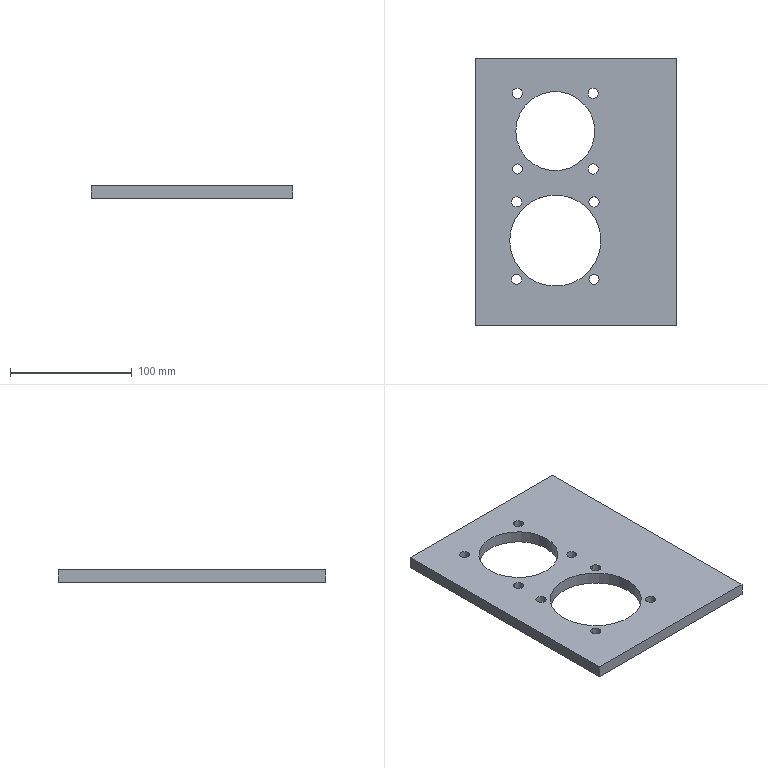Part | SolidWorks | features BaseBody 1 | 1 solid | 26 faces | box 166 x 220 x 10 mm | volume 283430 mm3 | cylinder 20 | plane 6 | commonest cylinder face diameters 8.376 x16 65 x2 75 x2
STEP:
#1=CARTESIAN_POINT('',(-32.665,-213.029,476.121));
#2=VERTEX_POINT('',#1);
#3=CARTESIAN_POINT('',(-107.665,-213.029,476.121));
#4=VERTEX_POINT('',#3);
#5=CARTESIAN_POINT('',(-70.165,-213.029,476.121));
#6=DIRECTION('',(0.,0.,-1.));
#7=DIRECTION('',(-1.,0.,0.));
#8=AXIS2_PLACEMENT_3D('',#5,#6,#7);
#9=CIRCLE('',#8,37.5);
#10=EDGE_CURVE('',#2,#4,#9,.T.);
#11=ORIENTED_EDGE('',*,*,#10,.F.);
#12=CARTESIAN_POINT('',(-32.665,-213.029,466.121));
#13=VERTEX_POINT('',#12);
#14=CARTESIAN_POINT('',(-32.665,-213.029,476.121));
#15=DIRECTION('',(0.,0.,-1.));
#16=VECTOR('',#15,1000.);
#17=LINE('',#14,#16);
#18=EDGE_CURVE('',#2,#13,#17,.T.);
#19=ORIENTED_EDGE('',*,*,#18,.T.);
#20=CARTESIAN_POINT('',(-107.665,-213.029,466.121));
#21=VERTEX_POINT('',#20);
#22=CARTESIAN_POINT('',(-70.165,-213.029,466.121));
#23=DIRECTION('',(0.,0.,-1.));
#24=DIRECTION('',(-1.,0.,0.));
#25=AXIS2_PLACEMENT_3D('',#22,#23,#24);
#26=CIRCLE('',#25,37.5);
#27=EDGE_CURVE('',#13,#21,#26,.T.);
#28=ORIENTED_EDGE('',*,*,#27,.T.);
#29=CARTESIAN_POINT('',(-107.665,-213.029,476.121));
#30=DIRECTION('',(0.,0.,-1.));
#31=VECTOR('',#30,1000.);
#32=LINE('',#29,#31);
#33=EDGE_CURVE('',#4,#21,#32,.T.);
#34=ORIENTED_EDGE('',*,*,#33,.F.);
#35=EDGE_LOOP('',(#11,#19,#28,#34));
#36=FACE_OUTER_BOUND('',#35,.T.);
#37=CARTESIAN_POINT('',(-70.165,-213.029,476.121));
#38=DIRECTION('',(0.,0.,-1.));
#39=DIRECTION('',(-1.,0.,0.));
#40=AXIS2_PLACEMENT_3D('',#37,#38,#39);
#41=CYLINDRICAL_SURFACE('',#40,37.5);
#42=ADVANCED_FACE('',(#36),#41,.F.);
#43=CARTESIAN_POINT('',(-37.665,-123.029,476.121));
#44=VERTEX_POINT('',#43);
#45=CARTESIAN_POINT('',(-102.665,-123.029,476.121));
#46=VERTEX_POINT('',#45);
#47=CARTESIAN_POINT('',(-70.165,-123.029,476.121));
#48=DIRECTION('',(0.,0.,-1.));
#49=DIRECTION('',(-1.,0.,0.));
#50=AXIS2_PLACEMENT_3D('',#47,#48,#49);
#51=CIRCLE('',#50,32.5);
#52=EDGE_CURVE('',#44,#46,#51,.T.);
#53=ORIENTED_EDGE('',*,*,#52,.F.);
#54=CARTESIAN_POINT('',(-37.665,-123.029,466.121));
#55=VERTEX_POINT('',#54);
#56=CARTESIAN_POINT('',(-37.665,-123.029,476.121));
#57=DIRECTION('',(0.,0.,-1.));
#58=VECTOR('',#57,1000.);
#59=LINE('',#56,#58);
#60=EDGE_CURVE('',#44,#55,#59,.T.);
#61=ORIENTED_EDGE('',*,*,#60,.T.);
#62=CARTESIAN_POINT('',(-102.665,-123.029,466.121));
#63=VERTEX_POINT('',#62);
#64=CARTESIAN_POINT('',(-70.165,-123.029,466.121));
#65=DIRECTION('',(0.,0.,-1.));
#66=DIRECTION('',(-1.,0.,0.));
#67=AXIS2_PLACEMENT_3D('',#64,#65,#66);
#68=CIRCLE('',#67,32.5);
#69=EDGE_CURVE('',#55,#63,#68,.T.);
#70=ORIENTED_EDGE('',*,*,#69,.T.);
#71=CARTESIAN_POINT('',(-102.665,-123.029,476.121));
#72=DIRECTION('',(0.,0.,-1.));
#73=VECTOR('',#72,1000.);
#74=LINE('',#71,#73);
#75=EDGE_CURVE('',#46,#63,#74,.T.);
#76=ORIENTED_EDGE('',*,*,#75,.F.);
#77=EDGE_LOOP('',(#53,#61,#70,#76));
#78=FACE_OUTER_BOUND('',#77,.T.);
#79=CARTESIAN_POINT('',(-70.165,-123.029,476.121));
#80=DIRECTION('',(0.,0.,-1.));
#81=DIRECTION('',(-1.,0.,0.));
#82=AXIS2_PLACEMENT_3D('',#79,#80,#81);
#83=CYLINDRICAL_SURFACE('',#82,32.5);
#84=ADVANCED_FACE('',(#78),#83,.F.);
#85=CARTESIAN_POINT('',(-39.052,-96.104,466.121));
#86=VERTEX_POINT('',#85);
#87=CARTESIAN_POINT('',(-39.052,-87.728,466.121));
#88=VERTEX_POINT('',#87);
#89=CARTESIAN_POINT('',(-39.052,-91.916,466.121));
#90=DIRECTION('',(0.,0.,-1.));
#91=DIRECTION('',(0.,-1.,0.));
#92=AXIS2_PLACEMENT_3D('',#89,#90,#91);
#93=CIRCLE('',#92,4.188);
#94=EDGE_CURVE('',#86,#88,#93,.T.);
#95=ORIENTED_EDGE('',*,*,#94,.T.);
#96=CARTESIAN_POINT('',(-39.052,-87.728,476.121));
#97=VERTEX_POINT('',#96);
#98=CARTESIAN_POINT('',(-39.052,-87.728,200.338));
#99=DIRECTION('',(0.,0.,1.));
#100=VECTOR('',#99,1000.);
#101=LINE('',#98,#100);
#102=EDGE_CURVE('',#88,#97,#101,.T.);
#103=ORIENTED_EDGE('',*,*,#102,.T.);
#104=CARTESIAN_POINT('',(-39.052,-96.104,476.121));
#105=VERTEX_POINT('',#104);
#106=CARTESIAN_POINT('',(-39.052,-91.916,476.121));
#107=DIRECTION('',(0.,0.,-1.));
#108=DIRECTION('',(0.,-1.,0.));
#109=AXIS2_PLACEMENT_3D('',#106,#107,#108);
#110=CIRCLE('',#109,4.188);
#111=EDGE_CURVE('',#105,#97,#110,.T.);
#112=ORIENTED_EDGE('',*,*,#111,.F.);
#113=CARTESIAN_POINT('',(-39.052,-96.104,200.338));
#114=DIRECTION('',(0.,0.,1.));
#115=VECTOR('',#114,1000.);
#116=LINE('',#113,#115);
#117=EDGE_CURVE('',#86,#105,#116,.T.);
#118=ORIENTED_EDGE('',*,*,#117,.F.);
#119=EDGE_LOOP('',(#95,#103,#112,#118));
#120=FACE_OUTER_BOUND('',#119,.T.);
#121=CARTESIAN_POINT('',(-39.052,-91.916,200.338));
#122=DIRECTION('',(0.,0.,1.));
#123=DIRECTION('',(0.,-1.,0.));
#124=AXIS2_PLACEMENT_3D('',#121,#122,#123);
#125=CYLINDRICAL_SURFACE('',#124,4.188);
#126=ADVANCED_FACE('',(#120),#125,.F.);
#127=CARTESIAN_POINT('',(-34.864,-154.141,466.121));
#128=VERTEX_POINT('',#127);
#129=CARTESIAN_POINT('',(-43.24,-154.141,466.121));
#130=VERTEX_POINT('',#129);
#131=CARTESIAN_POINT('',(-39.052,-154.141,466.121));
#132=DIRECTION('',(0.,0.,-1.));
#133=DIRECTION('',(1.,0.,0.));
#134=AXIS2_PLACEMENT_3D('',#131,#132,#133);
#135=CIRCLE('',#134,4.188);
#136=EDGE_CURVE('',#128,#130,#135,.T.);
#137=ORIENTED_EDGE('',*,*,#136,.T.);
#138=CARTESIAN_POINT('',(-43.24,-154.141,476.121));
#139=VERTEX_POINT('',#138);
#140=CARTESIAN_POINT('',(-43.24,-154.141,200.338));
#141=DIRECTION('',(0.,0.,1.));
#142=VECTOR('',#141,1000.);
#143=LINE('',#140,#142);
#144=EDGE_CURVE('',#130,#139,#143,.T.);
#145=ORIENTED_EDGE('',*,*,#144,.T.);
#146=CARTESIAN_POINT('',(-34.864,-154.141,476.121));
#147=VERTEX_POINT('',#146);
#148=CARTESIAN_POINT('',(-39.052,-154.141,476.121));
#149=DIRECTION('',(0.,0.,-1.));
#150=DIRECTION('',(1.,0.,0.));
#151=AXIS2_PLACEMENT_3D('',#148,#149,#150);
#152=CIRCLE('',#151,4.188);
#153=EDGE_CURVE('',#147,#139,#152,.T.);
#154=ORIENTED_EDGE('',*,*,#153,.F.);
#155=CARTESIAN_POINT('',(-34.864,-154.141,200.338));
#156=DIRECTION('',(0.,0.,1.));
#157=VECTOR('',#156,1000.);
#158=LINE('',#155,#157);
#159=EDGE_CURVE('',#128,#147,#158,.T.);
#160=ORIENTED_EDGE('',*,*,#159,.F.);
#161=EDGE_LOOP('',(#137,#145,#154,#160));
#162=FACE_OUTER_BOUND('',#161,.T.);
#163=CARTESIAN_POINT('',(-39.052,-154.141,200.338));
#164=DIRECTION('',(0.,0.,1.));
#165=DIRECTION('',(1.,0.,0.));
#166=AXIS2_PLACEMENT_3D('',#163,#164,#165);
#167=CYLINDRICAL_SURFACE('',#166,4.188);
#168=ADVANCED_FACE('',(#162),#167,.F.);
#169=CARTESIAN_POINT('',(-101.277,-158.329,466.121));
#170=VERTEX_POINT('',#169);
#171=CARTESIAN_POINT('',(-101.277,-149.953,466.121));
#172=VERTEX_POINT('',#171);
#173=CARTESIAN_POINT('',(-101.277,-154.141,466.121));
#174=DIRECTION('',(0.,0.,-1.));
#175=DIRECTION('',(0.,-1.,0.));
#176=AXIS2_PLACEMENT_3D('',#173,#174,#175);
#177=CIRCLE('',#176,4.188);
#178=EDGE_CURVE('',#170,#172,#177,.T.);
#179=ORIENTED_EDGE('',*,*,#178,.T.);
#180=CARTESIAN_POINT('',(-101.277,-149.953,476.121));
#181=VERTEX_POINT('',#180);
#182=CARTESIAN_POINT('',(-101.277,-149.953,200.338));
#183=DIRECTION('',(0.,0.,1.));
#184=VECTOR('',#183,1000.);
#185=LINE('',#182,#184);
#186=EDGE_CURVE('',#172,#181,#185,.T.);
#187=ORIENTED_EDGE('',*,*,#186,.T.);
#188=CARTESIAN_POINT('',(-101.277,-158.329,476.121));
#189=VERTEX_POINT('',#188);
#190=CARTESIAN_POINT('',(-101.277,-154.141,476.121));
#191=DIRECTION('',(0.,0.,-1.));
#192=DIRECTION('',(0.,-1.,0.));
#193=AXIS2_PLACEMENT_3D('',#190,#191,#192);
#194=CIRCLE('',#193,4.188);
#195=EDGE_CURVE('',#189,#181,#194,.T.);
#196=ORIENTED_EDGE('',*,*,#195,.F.);
#197=CARTESIAN_POINT('',(-101.277,-158.329,200.338));
#198=DIRECTION('',(0.,0.,1.));
#199=VECTOR('',#198,1000.);
#200=LINE('',#197,#199);
#201=EDGE_CURVE('',#170,#189,#200,.T.);
#202=ORIENTED_EDGE('',*,*,#201,.F.);
#203=EDGE_LOOP('',(#179,#187,#196,#202));
#204=FACE_OUTER_BOUND('',#203,.T.);
#205=CARTESIAN_POINT('',(-101.277,-154.141,200.338));
#206=DIRECTION('',(0.,0.,1.));
#207=DIRECTION('',(0.,-1.,0.));
#208=AXIS2_PLACEMENT_3D('',#205,#206,#207);
#209=CYLINDRICAL_SURFACE('',#208,4.188);
#210=ADVANCED_FACE('',(#204),#209,.F.);
#211=CARTESIAN_POINT('',(-97.089,-91.916,466.121));
#212=VERTEX_POINT('',#211);
#213=CARTESIAN_POINT('',(-105.465,-91.916,466.121));
#214=VERTEX_POINT('',#213);
#215=CARTESIAN_POINT('',(-101.277,-91.916,466.121));
#216=DIRECTION('',(0.,0.,-1.));
#217=DIRECTION('',(1.,0.,0.));
#218=AXIS2_PLACEMENT_3D('',#215,#216,#217);
#219=CIRCLE('',#218,4.188);
#220=EDGE_CURVE('',#212,#214,#219,.T.);
#221=ORIENTED_EDGE('',*,*,#220,.T.);
#222=CARTESIAN_POINT('',(-105.465,-91.916,476.121));
#223=VERTEX_POINT('',#222);
#224=CARTESIAN_POINT('',(-105.465,-91.916,200.338));
#225=DIRECTION('',(0.,0.,1.));
#226=VECTOR('',#225,1000.);
#227=LINE('',#224,#226);
#228=EDGE_CURVE('',#214,#223,#227,.T.);
#229=ORIENTED_EDGE('',*,*,#228,.T.);
#230=CARTESIAN_POINT('',(-97.089,-91.916,476.121));
#231=VERTEX_POINT('',#230);
#232=CARTESIAN_POINT('',(-101.277,-91.916,476.121));
#233=DIRECTION('',(0.,0.,-1.));
#234=DIRECTION('',(1.,0.,0.));
#235=AXIS2_PLACEMENT_3D('',#232,#233,#234);
#236=CIRCLE('',#235,4.188);
#237=EDGE_CURVE('',#231,#223,#236,.T.);
#238=ORIENTED_EDGE('',*,*,#237,.F.);
#239=CARTESIAN_POINT('',(-97.089,-91.916,200.338));
#240=DIRECTION('',(0.,0.,1.));
#241=VECTOR('',#240,1000.);
#242=LINE('',#239,#241);
#243=EDGE_CURVE('',#212,#231,#242,.T.);
#244=ORIENTED_EDGE('',*,*,#243,.F.);
#245=EDGE_LOOP('',(#221,#229,#238,#244));
#246=FACE_OUTER_BOUND('',#245,.T.);
#247=CARTESIAN_POINT('',(-101.277,-91.916,200.338));
#248=DIRECTION('',(0.,0.,1.));
#249=DIRECTION('',(1.,0.,0.));
#250=AXIS2_PLACEMENT_3D('',#247,#248,#249);
#251=CYLINDRICAL_SURFACE('',#250,4.188);
#252=ADVANCED_FACE('',(#246),#251,.F.);
#253=CARTESIAN_POINT('',(-38.345,-185.397,466.121));
#254=VERTEX_POINT('',#253);
#255=CARTESIAN_POINT('',(-38.345,-177.021,466.121));
#256=VERTEX_POINT('',#255);
#257=CARTESIAN_POINT('',(-38.345,-181.209,466.121));
#258=DIRECTION('',(0.,0.,-1.));
#259=DIRECTION('',(0.,-1.,0.));
#260=AXIS2_PLACEMENT_3D('',#257,#258,#259);
#261=CIRCLE('',#260,4.188);
#262=EDGE_CURVE('',#254,#256,#261,.T.);
#263=ORIENTED_EDGE('',*,*,#262,.T.);
#264=CARTESIAN_POINT('',(-38.345,-177.021,476.121));
#265=VERTEX_POINT('',#264);
#266=CARTESIAN_POINT('',(-38.345,-177.021,200.338));
#267=DIRECTION('',(0.,0.,1.));
#268=VECTOR('',#267,1000.);
#269=LINE('',#266,#268);
#270=EDGE_CURVE('',#256,#265,#269,.T.);
#271=ORIENTED_EDGE('',*,*,#270,.T.);
#272=CARTESIAN_POINT('',(-38.345,-185.397,476.121));
#273=VERTEX_POINT('',#272);
#274=CARTESIAN_POINT('',(-38.345,-181.209,476.121));
#275=DIRECTION('',(0.,0.,-1.));
#276=DIRECTION('',(0.,-1.,0.));
#277=AXIS2_PLACEMENT_3D('',#274,#275,#276);
#278=CIRCLE('',#277,4.188);
#279=EDGE_CURVE('',#273,#265,#278,.T.);
#280=ORIENTED_EDGE('',*,*,#279,.F.);
#281=CARTESIAN_POINT('',(-38.345,-185.397,200.338));
#282=DIRECTION('',(0.,0.,1.));
#283=VECTOR('',#282,1000.);
#284=LINE('',#281,#283);
#285=EDGE_CURVE('',#254,#273,#284,.T.);
#286=ORIENTED_EDGE('',*,*,#285,.F.);
#287=EDGE_LOOP('',(#263,#271,#280,#286));
#288=FACE_OUTER_BOUND('',#287,.T.);
#289=CARTESIAN_POINT('',(-38.345,-181.209,200.338));
#290=DIRECTION('',(0.,0.,1.));
#291=DIRECTION('',(0.,-1.,0.));
#292=AXIS2_PLACEMENT_3D('',#289,#290,#291);
#293=CYLINDRICAL_SURFACE('',#292,4.188);
#294=ADVANCED_FACE('',(#288),#293,.F.);
#295=CARTESIAN_POINT('',(-34.157,-244.848,466.121));
#296=VERTEX_POINT('',#295);
#297=CARTESIAN_POINT('',(-42.533,-244.848,466.121));
#298=VERTEX_POINT('',#297);
#299=CARTESIAN_POINT('',(-38.345,-244.848,466.121));
#300=DIRECTION('',(0.,0.,-1.));
#301=DIRECTION('',(1.,0.,0.));
#302=AXIS2_PLACEMENT_3D('',#299,#300,#301);
#303=CIRCLE('',#302,4.188);
#304=EDGE_CURVE('',#296,#298,#303,.T.);
#305=ORIENTED_EDGE('',*,*,#304,.T.);
#306=CARTESIAN_POINT('',(-42.533,-244.848,476.121));
#307=VERTEX_POINT('',#306);
#308=CARTESIAN_POINT('',(-42.533,-244.848,200.338));
#309=DIRECTION('',(0.,0.,1.));
#310=VECTOR('',#309,1000.);
#311=LINE('',#308,#310);
#312=EDGE_CURVE('',#298,#307,#311,.T.);
#313=ORIENTED_EDGE('',*,*,#312,.T.);
#314=CARTESIAN_POINT('',(-34.157,-244.848,476.121));
#315=VERTEX_POINT('',#314);
#316=CARTESIAN_POINT('',(-38.345,-244.848,476.121));
#317=DIRECTION('',(0.,0.,-1.));
#318=DIRECTION('',(1.,0.,0.));
#319=AXIS2_PLACEMENT_3D('',#316,#317,#318);
#320=CIRCLE('',#319,4.188);
#321=EDGE_CURVE('',#315,#307,#320,.T.);
#322=ORIENTED_EDGE('',*,*,#321,.F.);
#323=CARTESIAN_POINT('',(-34.157,-244.848,200.338));
#324=DIRECTION('',(0.,0.,1.));
#325=VECTOR('',#324,1000.);
#326=LINE('',#323,#325);
#327=EDGE_CURVE('',#296,#315,#326,.T.);
#328=ORIENTED_EDGE('',*,*,#327,.F.);
#329=EDGE_LOOP('',(#305,#313,#322,#328));
#330=FACE_OUTER_BOUND('',#329,.T.);
#331=CARTESIAN_POINT('',(-38.345,-244.848,200.338));
#332=DIRECTION('',(0.,0.,1.));
#333=DIRECTION('',(1.,0.,0.));
#334=AXIS2_PLACEMENT_3D('',#331,#332,#333);
#335=CYLINDRICAL_SURFACE('',#334,4.188);
#336=ADVANCED_FACE('',(#330),#335,.F.);
#337=CARTESIAN_POINT('',(-101.984,-249.036,466.121));
#338=VERTEX_POINT('',#337);
#339=CARTESIAN_POINT('',(-101.984,-240.66,466.121));
#340=VERTEX_POINT('',#339);
#341=CARTESIAN_POINT('',(-101.984,-244.848,466.121));
#342=DIRECTION('',(0.,0.,-1.));
#343=DIRECTION('',(0.,-1.,0.));
#344=AXIS2_PLACEMENT_3D('',#341,#342,#343);
#345=CIRCLE('',#344,4.188);
#346=EDGE_CURVE('',#338,#340,#345,.T.);
#347=ORIENTED_EDGE('',*,*,#346,.T.);
#348=CARTESIAN_POINT('',(-101.984,-240.66,476.121));
#349=VERTEX_POINT('',#348);
#350=CARTESIAN_POINT('',(-101.984,-240.66,200.338));
#351=DIRECTION('',(0.,0.,1.));
#352=VECTOR('',#351,1000.);
#353=LINE('',#350,#352);
#354=EDGE_CURVE('',#340,#349,#353,.T.);
#355=ORIENTED_EDGE('',*,*,#354,.T.);
#356=CARTESIAN_POINT('',(-101.984,-249.036,476.121));
#357=VERTEX_POINT('',#356);
#358=CARTESIAN_POINT('',(-101.984,-244.848,476.121));
#359=DIRECTION('',(0.,0.,-1.));
#360=DIRECTION('',(0.,-1.,0.));
#361=AXIS2_PLACEMENT_3D('',#358,#359,#360);
#362=CIRCLE('',#361,4.188);
#363=EDGE_CURVE('',#357,#349,#362,.T.);
#364=ORIENTED_EDGE('',*,*,#363,.F.);
#365=CARTESIAN_POINT('',(-101.984,-249.036,200.338));
#366=DIRECTION('',(0.,0.,1.));
#367=VECTOR('',#366,1000.);
#368=LINE('',#365,#367);
#369=EDGE_CURVE('',#338,#357,#368,.T.);
#370=ORIENTED_EDGE('',*,*,#369,.F.);
#371=EDGE_LOOP('',(#347,#355,#364,#370));
#372=FACE_OUTER_BOUND('',#371,.T.);
#373=CARTESIAN_POINT('',(-101.984,-244.848,200.338));
#374=DIRECTION('',(0.,0.,1.));
#375=DIRECTION('',(0.,-1.,0.));
#376=AXIS2_PLACEMENT_3D('',#373,#374,#375);
#377=CYLINDRICAL_SURFACE('',#376,4.188);
#378=ADVANCED_FACE('',(#372),#377,.F.);
#379=CARTESIAN_POINT('',(-97.796,-181.209,466.121));
#380=VERTEX_POINT('',#379);
#381=CARTESIAN_POINT('',(-106.172,-181.209,466.121));
#382=VERTEX_POINT('',#381);
#383=CARTESIAN_POINT('',(-101.984,-181.209,466.121));
#384=DIRECTION('',(0.,0.,-1.));
#385=DIRECTION('',(1.,0.,0.));
#386=AXIS2_PLACEMENT_3D('',#383,#384,#385);
#387=CIRCLE('',#386,4.188);
#388=EDGE_CURVE('',#380,#382,#387,.T.);
#389=ORIENTED_EDGE('',*,*,#388,.T.);
#390=CARTESIAN_POINT('',(-106.172,-181.209,476.121));
#391=VERTEX_POINT('',#390);
#392=CARTESIAN_POINT('',(-106.172,-181.209,200.338));
#393=DIRECTION('',(0.,0.,1.));
#394=VECTOR('',#393,1000.);
#395=LINE('',#392,#394);
#396=EDGE_CURVE('',#382,#391,#395,.T.);
#397=ORIENTED_EDGE('',*,*,#396,.T.);
#398=CARTESIAN_POINT('',(-97.796,-181.209,476.121));
#399=VERTEX_POINT('',#398);
#400=CARTESIAN_POINT('',(-101.984,-181.209,476.121));
#401=DIRECTION('',(0.,0.,-1.));
#402=DIRECTION('',(1.,0.,0.));
#403=AXIS2_PLACEMENT_3D('',#400,#401,#402);
#404=CIRCLE('',#403,4.188);
#405=EDGE_CURVE('',#399,#391,#404,.T.);
#406=ORIENTED_EDGE('',*,*,#405,.F.);
#407=CARTESIAN_POINT('',(-97.796,-181.209,200.338));
#408=DIRECTION('',(0.,0.,1.));
#409=VECTOR('',#408,1000.);
#410=LINE('',#407,#409);
#411=EDGE_CURVE('',#380,#399,#410,.T.);
#412=ORIENTED_EDGE('',*,*,#411,.F.);
#413=EDGE_LOOP('',(#389,#397,#406,#412));
#414=FACE_OUTER_BOUND('',#413,.T.);
#415=CARTESIAN_POINT('',(-101.984,-181.209,200.338));
#416=DIRECTION('',(0.,0.,1.));
#417=DIRECTION('',(1.,0.,0.));
#418=AXIS2_PLACEMENT_3D('',#415,#416,#417);
#419=CYLINDRICAL_SURFACE('',#418,4.188);
#420=ADVANCED_FACE('',(#414),#419,.F.);
#421=CARTESIAN_POINT('',(-70.165,-213.029,466.121));
#422=DIRECTION('',(0.,0.,-1.));
#423=DIRECTION('',(-1.,0.,0.));
#424=AXIS2_PLACEMENT_3D('',#421,#422,#423);
#425=CIRCLE('',#424,37.5);
#426=EDGE_CURVE('',#21,#13,#425,.T.);
#427=ORIENTED_EDGE('',*,*,#426,.F.);
#428=ORIENTED_EDGE('',*,*,#27,.F.);
#429=EDGE_LOOP('',(#427,#428));
#430=FACE_BOUND('',#429,.T.);
#431=CARTESIAN_POINT('',(-70.165,-123.029,466.121));
#432=DIRECTION('',(0.,0.,-1.));
#433=DIRECTION('',(-1.,0.,0.));
#434=AXIS2_PLACEMENT_3D('',#431,#432,#433);
#435=CIRCLE('',#434,32.5);
#436=EDGE_CURVE('',#63,#55,#435,.T.);
#437=ORIENTED_EDGE('',*,*,#436,.F.);
#438=ORIENTED_EDGE('',*,*,#69,.F.);
#439=EDGE_LOOP('',(#437,#438));
#440=FACE_BOUND('',#439,.T.);
#441=ORIENTED_EDGE('',*,*,#94,.F.);
#442=CARTESIAN_POINT('',(-39.052,-91.916,466.121));
#443=DIRECTION('',(0.,0.,-1.));
#444=DIRECTION('',(0.,-1.,0.));
#445=AXIS2_PLACEMENT_3D('',#442,#443,#444);
#446=CIRCLE('',#445,4.188);
#447=EDGE_CURVE('',#88,#86,#446,.T.);
#448=ORIENTED_EDGE('',*,*,#447,.F.);
#449=EDGE_LOOP('',(#441,#448));
#450=FACE_BOUND('',#449,.T.);
#451=ORIENTED_EDGE('',*,*,#136,.F.);
#452=CARTESIAN_POINT('',(-39.052,-154.141,466.121));
#453=DIRECTION('',(0.,0.,-1.));
#454=DIRECTION('',(1.,0.,0.));
#455=AXIS2_PLACEMENT_3D('',#452,#453,#454);
#456=CIRCLE('',#455,4.188);
#457=EDGE_CURVE('',#130,#128,#456,.T.);
#458=ORIENTED_EDGE('',*,*,#457,.F.);
#459=EDGE_LOOP('',(#451,#458));
#460=FACE_BOUND('',#459,.T.);
#461=ORIENTED_EDGE('',*,*,#178,.F.);
#462=CARTESIAN_POINT('',(-101.277,-154.141,466.121));
#463=DIRECTION('',(0.,0.,-1.));
#464=DIRECTION('',(0.,-1.,0.));
#465=AXIS2_PLACEMENT_3D('',#462,#463,#464);
#466=CIRCLE('',#465,4.188);
#467=EDGE_CURVE('',#172,#170,#466,.T.);
#468=ORIENTED_EDGE('',*,*,#467,.F.);
#469=EDGE_LOOP('',(#461,#468));
#470=FACE_BOUND('',#469,.T.);
#471=ORIENTED_EDGE('',*,*,#220,.F.);
#472=CARTESIAN_POINT('',(-101.277,-91.916,466.121));
#473=DIRECTION('',(0.,0.,-1.));
#474=DIRECTION('',(1.,0.,0.));
#475=AXIS2_PLACEMENT_3D('',#472,#473,#474);
#476=CIRCLE('',#475,4.188);
#477=EDGE_CURVE('',#214,#212,#476,.T.);
#478=ORIENTED_EDGE('',*,*,#477,.F.);
#479=EDGE_LOOP('',(#471,#478));
#480=FACE_BOUND('',#479,.T.);
#481=ORIENTED_EDGE('',*,*,#262,.F.);
#482=CARTESIAN_POINT('',(-38.345,-181.209,466.121));
#483=DIRECTION('',(0.,0.,-1.));
#484=DIRECTION('',(0.,-1.,0.));
#485=AXIS2_PLACEMENT_3D('',#482,#483,#484);
#486=CIRCLE('',#485,4.188);
#487=EDGE_CURVE('',#256,#254,#486,.T.);
#488=ORIENTED_EDGE('',*,*,#487,.F.);
#489=EDGE_LOOP('',(#481,#488));
#490=FACE_BOUND('',#489,.T.);
#491=ORIENTED_EDGE('',*,*,#304,.F.);
#492=CARTESIAN_POINT('',(-38.345,-244.848,466.121));
#493=DIRECTION('',(0.,0.,-1.));
#494=DIRECTION('',(1.,0.,0.));
#495=AXIS2_PLACEMENT_3D('',#492,#493,#494);
#496=CIRCLE('',#495,4.188);
#497=EDGE_CURVE('',#298,#296,#496,.T.);
#498=ORIENTED_EDGE('',*,*,#497,.F.);
#499=EDGE_LOOP('',(#491,#498));
#500=FACE_BOUND('',#499,.T.);
#501=ORIENTED_EDGE('',*,*,#346,.F.);
#502=CARTESIAN_POINT('',(-101.984,-244.848,466.121));
#503=DIRECTION('',(0.,0.,-1.));
#504=DIRECTION('',(0.,-1.,0.));
#505=AXIS2_PLACEMENT_3D('',#502,#503,#504);
#506=CIRCLE('',#505,4.188);
#507=EDGE_CURVE('',#340,#338,#506,.T.);
#508=ORIENTED_EDGE('',*,*,#507,.F.);
#509=EDGE_LOOP('',(#501,#508));
#510=FACE_BOUND('',#509,.T.);
#511=ORIENTED_EDGE('',*,*,#388,.F.);
#512=CARTESIAN_POINT('',(-101.984,-181.209,466.121));
#513=DIRECTION('',(0.,0.,-1.));
#514=DIRECTION('',(1.,0.,0.));
#515=AXIS2_PLACEMENT_3D('',#512,#513,#514);
#516=CIRCLE('',#515,4.188);
#517=EDGE_CURVE('',#382,#380,#516,.T.);
#518=ORIENTED_EDGE('',*,*,#517,.F.);
#519=EDGE_LOOP('',(#511,#518));
#520=FACE_BOUND('',#519,.T.);
#521=CARTESIAN_POINT('',(-136.165,-283.029,466.121));
#522=VERTEX_POINT('',#521);
#523=CARTESIAN_POINT('',(29.835,-283.029,466.121));
#524=VERTEX_POINT('',#523);
#525=CARTESIAN_POINT('',(-53.165,-283.029,466.121));
#526=DIRECTION('',(1.,0.,0.));
#527=VECTOR('',#526,1000.);
#528=LINE('',#525,#527);
#529=EDGE_CURVE('',#522,#524,#528,.T.);
#530=ORIENTED_EDGE('',*,*,#529,.F.);
#531=CARTESIAN_POINT('',(-136.165,-63.029,466.121));
#532=VERTEX_POINT('',#531);
#533=CARTESIAN_POINT('',(-136.165,-173.029,466.121));
#534=DIRECTION('',(0.,-1.,0.));
#535=VECTOR('',#534,1000.);
#536=LINE('',#533,#535);
#537=EDGE_CURVE('',#532,#522,#536,.T.);
#538=ORIENTED_EDGE('',*,*,#537,.F.);
#539=CARTESIAN_POINT('',(29.835,-63.029,466.121));
#540=VERTEX_POINT('',#539);
#541=CARTESIAN_POINT('',(-53.165,-63.029,466.121));
#542=DIRECTION('',(-1.,0.,0.));
#543=VECTOR('',#542,1000.);
#544=LINE('',#541,#543);
#545=EDGE_CURVE('',#540,#532,#544,.T.);
#546=ORIENTED_EDGE('',*,*,#545,.F.);
#547=CARTESIAN_POINT('',(29.835,-173.029,466.121));
#548=DIRECTION('',(0.,1.,0.));
#549=VECTOR('',#548,1000.);
#550=LINE('',#547,#549);
#551=EDGE_CURVE('',#524,#540,#550,.T.);
#552=ORIENTED_EDGE('',*,*,#551,.F.);
#553=EDGE_LOOP('',(#530,#538,#546,#552));
#554=FACE_OUTER_BOUND('',#553,.T.);
#555=CARTESIAN_POINT('',(-53.165,-173.029,466.121));
#556=DIRECTION('',(0.,0.,1.));
#557=DIRECTION('',(0.,-1.,0.));
#558=AXIS2_PLACEMENT_3D('',#555,#556,#557);
#559=PLANE('',#558);
#560=ADVANCED_FACE('',(#430,#440,#450,#460,#470,#480,#490,#500,#510,#520,#554),#559,.F.);
#561=ORIENTED_EDGE('',*,*,#18,.F.);
#562=CARTESIAN_POINT('',(-70.165,-213.029,476.121));
#563=DIRECTION('',(0.,0.,-1.));
#564=DIRECTION('',(-1.,0.,0.));
#565=AXIS2_PLACEMENT_3D('',#562,#563,#564);
#566=CIRCLE('',#565,37.5);
#567=EDGE_CURVE('',#4,#2,#566,.T.);
#568=ORIENTED_EDGE('',*,*,#567,.F.);
#569=ORIENTED_EDGE('',*,*,#33,.T.);
#570=ORIENTED_EDGE('',*,*,#426,.T.);
#571=EDGE_LOOP('',(#561,#568,#569,#570));
#572=FACE_OUTER_BOUND('',#571,.T.);
#573=CARTESIAN_POINT('',(-70.165,-213.029,476.121));
#574=DIRECTION('',(0.,0.,-1.));
#575=DIRECTION('',(-1.,0.,0.));
#576=AXIS2_PLACEMENT_3D('',#573,#574,#575);
#577=CYLINDRICAL_SURFACE('',#576,37.5);
#578=ADVANCED_FACE('',(#572),#577,.F.);
#579=ORIENTED_EDGE('',*,*,#60,.F.);
#580=CARTESIAN_POINT('',(-70.165,-123.029,476.121));
#581=DIRECTION('',(0.,0.,-1.));
#582=DIRECTION('',(-1.,0.,0.));
#583=AXIS2_PLACEMENT_3D('',#580,#581,#582);
#584=CIRCLE('',#583,32.5);
#585=EDGE_CURVE('',#46,#44,#584,.T.);
#586=ORIENTED_EDGE('',*,*,#585,.F.);
#587=ORIENTED_EDGE('',*,*,#75,.T.);
#588=ORIENTED_EDGE('',*,*,#436,.T.);
#589=EDGE_LOOP('',(#579,#586,#587,#588));
#590=FACE_OUTER_BOUND('',#589,.T.);
#591=CARTESIAN_POINT('',(-70.165,-123.029,476.121));
#592=DIRECTION('',(0.,0.,-1.));
#593=DIRECTION('',(-1.,0.,0.));
#594=AXIS2_PLACEMENT_3D('',#591,#592,#593);
#595=CYLINDRICAL_SURFACE('',#594,32.5);
#596=ADVANCED_FACE('',(#590),#595,.F.);
#597=ORIENTED_EDGE('',*,*,#102,.F.);
#598=ORIENTED_EDGE('',*,*,#447,.T.);
#599=ORIENTED_EDGE('',*,*,#117,.T.);
#600=CARTESIAN_POINT('',(-39.052,-91.916,476.121));
#601=DIRECTION('',(0.,0.,-1.));
#602=DIRECTION('',(0.,-1.,0.));
#603=AXIS2_PLACEMENT_3D('',#600,#601,#602);
#604=CIRCLE('',#603,4.188);
#605=EDGE_CURVE('',#97,#105,#604,.T.);
#606=ORIENTED_EDGE('',*,*,#605,.F.);
#607=EDGE_LOOP('',(#597,#598,#599,#606));
#608=FACE_OUTER_BOUND('',#607,.T.);
#609=CARTESIAN_POINT('',(-39.052,-91.916,200.338));
#610=DIRECTION('',(0.,0.,1.));
#611=DIRECTION('',(0.,-1.,0.));
#612=AXIS2_PLACEMENT_3D('',#609,#610,#611);
#613=CYLINDRICAL_SURFACE('',#612,4.188);
#614=ADVANCED_FACE('',(#608),#613,.F.);
#615=ORIENTED_EDGE('',*,*,#144,.F.);
#616=ORIENTED_EDGE('',*,*,#457,.T.);
#617=ORIENTED_EDGE('',*,*,#159,.T.);
#618=CARTESIAN_POINT('',(-39.052,-154.141,476.121));
#619=DIRECTION('',(0.,0.,-1.));
#620=DIRECTION('',(1.,0.,0.));
#621=AXIS2_PLACEMENT_3D('',#618,#619,#620);
#622=CIRCLE('',#621,4.188);
#623=EDGE_CURVE('',#139,#147,#622,.T.);
#624=ORIENTED_EDGE('',*,*,#623,.F.);
#625=EDGE_LOOP('',(#615,#616,#617,#624));
#626=FACE_OUTER_BOUND('',#625,.T.);
#627=CARTESIAN_POINT('',(-39.052,-154.141,200.338));
#628=DIRECTION('',(0.,0.,1.));
#629=DIRECTION('',(1.,0.,0.));
#630=AXIS2_PLACEMENT_3D('',#627,#628,#629);
#631=CYLINDRICAL_SURFACE('',#630,4.188);
#632=ADVANCED_FACE('',(#626),#631,.F.);
#633=ORIENTED_EDGE('',*,*,#186,.F.);
#634=ORIENTED_EDGE('',*,*,#467,.T.);
#635=ORIENTED_EDGE('',*,*,#201,.T.);
#636=CARTESIAN_POINT('',(-101.277,-154.141,476.121));
#637=DIRECTION('',(0.,0.,-1.));
#638=DIRECTION('',(0.,-1.,0.));
#639=AXIS2_PLACEMENT_3D('',#636,#637,#638);
#640=CIRCLE('',#639,4.188);
#641=EDGE_CURVE('',#181,#189,#640,.T.);
#642=ORIENTED_EDGE('',*,*,#641,.F.);
#643=EDGE_LOOP('',(#633,#634,#635,#642));
#644=FACE_OUTER_BOUND('',#643,.T.);
#645=CARTESIAN_POINT('',(-101.277,-154.141,200.338));
#646=DIRECTION('',(0.,0.,1.));
#647=DIRECTION('',(0.,-1.,0.));
#648=AXIS2_PLACEMENT_3D('',#645,#646,#647);
#649=CYLINDRICAL_SURFACE('',#648,4.188);
#650=ADVANCED_FACE('',(#644),#649,.F.);
#651=ORIENTED_EDGE('',*,*,#228,.F.);
#652=ORIENTED_EDGE('',*,*,#477,.T.);
#653=ORIENTED_EDGE('',*,*,#243,.T.);
#654=CARTESIAN_POINT('',(-101.277,-91.916,476.121));
#655=DIRECTION('',(0.,0.,-1.));
#656=DIRECTION('',(1.,0.,0.));
#657=AXIS2_PLACEMENT_3D('',#654,#655,#656);
#658=CIRCLE('',#657,4.188);
#659=EDGE_CURVE('',#223,#231,#658,.T.);
#660=ORIENTED_EDGE('',*,*,#659,.F.);
#661=EDGE_LOOP('',(#651,#652,#653,#660));
#662=FACE_OUTER_BOUND('',#661,.T.);
#663=CARTESIAN_POINT('',(-101.277,-91.916,200.338));
#664=DIRECTION('',(0.,0.,1.));
#665=DIRECTION('',(1.,0.,0.));
#666=AXIS2_PLACEMENT_3D('',#663,#664,#665);
#667=CYLINDRICAL_SURFACE('',#666,4.188);
#668=ADVANCED_FACE('',(#662),#667,.F.);
#669=ORIENTED_EDGE('',*,*,#270,.F.);
#670=ORIENTED_EDGE('',*,*,#487,.T.);
#671=ORIENTED_EDGE('',*,*,#285,.T.);
#672=CARTESIAN_POINT('',(-38.345,-181.209,476.121));
#673=DIRECTION('',(0.,0.,-1.));
#674=DIRECTION('',(0.,-1.,0.));
#675=AXIS2_PLACEMENT_3D('',#672,#673,#674);
#676=CIRCLE('',#675,4.188);
#677=EDGE_CURVE('',#265,#273,#676,.T.);
#678=ORIENTED_EDGE('',*,*,#677,.F.);
#679=EDGE_LOOP('',(#669,#670,#671,#678));
#680=FACE_OUTER_BOUND('',#679,.T.);
#681=CARTESIAN_POINT('',(-38.345,-181.209,200.338));
#682=DIRECTION('',(0.,0.,1.));
#683=DIRECTION('',(0.,-1.,0.));
#684=AXIS2_PLACEMENT_3D('',#681,#682,#683);
#685=CYLINDRICAL_SURFACE('',#684,4.188);
#686=ADVANCED_FACE('',(#680),#685,.F.);
#687=ORIENTED_EDGE('',*,*,#312,.F.);
#688=ORIENTED_EDGE('',*,*,#497,.T.);
#689=ORIENTED_EDGE('',*,*,#327,.T.);
#690=CARTESIAN_POINT('',(-38.345,-244.848,476.121));
#691=DIRECTION('',(0.,0.,-1.));
#692=DIRECTION('',(1.,0.,0.));
#693=AXIS2_PLACEMENT_3D('',#690,#691,#692);
#694=CIRCLE('',#693,4.188);
#695=EDGE_CURVE('',#307,#315,#694,.T.);
#696=ORIENTED_EDGE('',*,*,#695,.F.);
#697=EDGE_LOOP('',(#687,#688,#689,#696));
#698=FACE_OUTER_BOUND('',#697,.T.);
#699=CARTESIAN_POINT('',(-38.345,-244.848,200.338));
#700=DIRECTION('',(0.,0.,1.));
#701=DIRECTION('',(1.,0.,0.));
#702=AXIS2_PLACEMENT_3D('',#699,#700,#701);
#703=CYLINDRICAL_SURFACE('',#702,4.188);
#704=ADVANCED_FACE('',(#698),#703,.F.);
#705=ORIENTED_EDGE('',*,*,#354,.F.);
#706=ORIENTED_EDGE('',*,*,#507,.T.);
#707=ORIENTED_EDGE('',*,*,#369,.T.);
#708=CARTESIAN_POINT('',(-101.984,-244.848,476.121));
#709=DIRECTION('',(0.,0.,-1.));
#710=DIRECTION('',(0.,-1.,0.));
#711=AXIS2_PLACEMENT_3D('',#708,#709,#710);
#712=CIRCLE('',#711,4.188);
#713=EDGE_CURVE('',#349,#357,#712,.T.);
#714=ORIENTED_EDGE('',*,*,#713,.F.);
#715=EDGE_LOOP('',(#705,#706,#707,#714));
#716=FACE_OUTER_BOUND('',#715,.T.);
#717=CARTESIAN_POINT('',(-101.984,-244.848,200.338));
#718=DIRECTION('',(0.,0.,1.));
#719=DIRECTION('',(0.,-1.,0.));
#720=AXIS2_PLACEMENT_3D('',#717,#718,#719);
#721=CYLINDRICAL_SURFACE('',#720,4.188);
#722=ADVANCED_FACE('',(#716),#721,.F.);
#723=ORIENTED_EDGE('',*,*,#396,.F.);
#724=ORIENTED_EDGE('',*,*,#517,.T.);
#725=ORIENTED_EDGE('',*,*,#411,.T.);
#726=CARTESIAN_POINT('',(-101.984,-181.209,476.121));
#727=DIRECTION('',(0.,0.,-1.));
#728=DIRECTION('',(1.,0.,0.));
#729=AXIS2_PLACEMENT_3D('',#726,#727,#728);
#730=CIRCLE('',#729,4.188);
#731=EDGE_CURVE('',#391,#399,#730,.T.);
#732=ORIENTED_EDGE('',*,*,#731,.F.);
#733=EDGE_LOOP('',(#723,#724,#725,#732));
#734=FACE_OUTER_BOUND('',#733,.T.);
#735=CARTESIAN_POINT('',(-101.984,-181.209,200.338));
#736=DIRECTION('',(0.,0.,1.));
#737=DIRECTION('',(1.,0.,0.));
#738=AXIS2_PLACEMENT_3D('',#735,#736,#737);
#739=CYLINDRICAL_SURFACE('',#738,4.188);
#740=ADVANCED_FACE('',(#734),#739,.F.);
#741=ORIENTED_EDGE('',*,*,#551,.T.);
#742=CARTESIAN_POINT('',(29.835,-63.029,476.121));
#743=VERTEX_POINT('',#742);
#744=CARTESIAN_POINT('',(29.835,-63.029,466.121));
#745=DIRECTION('',(0.,0.,1.));
#746=VECTOR('',#745,1000.);
#747=LINE('',#744,#746);
#748=EDGE_CURVE('',#540,#743,#747,.T.);
#749=ORIENTED_EDGE('',*,*,#748,.T.);
#750=CARTESIAN_POINT('',(29.835,-283.029,476.121));
#751=VERTEX_POINT('',#750);
#752=CARTESIAN_POINT('',(29.835,-63.029,476.121));
#753=DIRECTION('',(0.,-1.,0.));
#754=VECTOR('',#753,1000.);
#755=LINE('',#752,#754);
#756=EDGE_CURVE('',#743,#751,#755,.T.);
#757=ORIENTED_EDGE('',*,*,#756,.T.);
#758=CARTESIAN_POINT('',(29.835,-283.029,466.121));
#759=DIRECTION('',(0.,0.,-1.));
#760=VECTOR('',#759,1000.);
#761=LINE('',#758,#760);
#762=EDGE_CURVE('',#751,#524,#761,.T.);
#763=ORIENTED_EDGE('',*,*,#762,.T.);
#764=EDGE_LOOP('',(#741,#749,#757,#763));
#765=FACE_OUTER_BOUND('',#764,.T.);
#766=CARTESIAN_POINT('',(29.835,-63.029,466.121));
#767=DIRECTION('',(1.,0.,0.));
#768=DIRECTION('',(0.,0.,-1.));
#769=AXIS2_PLACEMENT_3D('',#766,#767,#768);
#770=PLANE('',#769);
#771=ADVANCED_FACE('',(#765),#770,.T.);
#772=ORIENTED_EDGE('',*,*,#529,.T.);
#773=ORIENTED_EDGE('',*,*,#762,.F.);
#774=CARTESIAN_POINT('',(-136.165,-283.029,476.121));
#775=VERTEX_POINT('',#774);
#776=CARTESIAN_POINT('',(29.835,-283.029,476.121));
#777=DIRECTION('',(-1.,0.,0.));
#778=VECTOR('',#777,1000.);
#779=LINE('',#776,#778);
#780=EDGE_CURVE('',#751,#775,#779,.T.);
#781=ORIENTED_EDGE('',*,*,#780,.T.);
#782=CARTESIAN_POINT('',(-136.165,-283.029,466.121));
#783=DIRECTION('',(0.,0.,-1.));
#784=VECTOR('',#783,1000.);
#785=LINE('',#782,#784);
#786=EDGE_CURVE('',#775,#522,#785,.T.);
#787=ORIENTED_EDGE('',*,*,#786,.T.);
#788=EDGE_LOOP('',(#772,#773,#781,#787));
#789=FACE_OUTER_BOUND('',#788,.T.);
#790=CARTESIAN_POINT('',(29.835,-283.029,466.121));
#791=DIRECTION('',(0.,-1.,0.));
#792=DIRECTION('',(0.,0.,-1.));
#793=AXIS2_PLACEMENT_3D('',#790,#791,#792);
#794=PLANE('',#793);
#795=ADVANCED_FACE('',(#789),#794,.T.);
#796=ORIENTED_EDGE('',*,*,#537,.T.);
#797=ORIENTED_EDGE('',*,*,#786,.F.);
#798=CARTESIAN_POINT('',(-136.165,-63.029,476.121));
#799=VERTEX_POINT('',#798);
#800=CARTESIAN_POINT('',(-136.165,-283.029,476.121));
#801=DIRECTION('',(0.,1.,0.));
#802=VECTOR('',#801,1000.);
#803=LINE('',#800,#802);
#804=EDGE_CURVE('',#775,#799,#803,.T.);
#805=ORIENTED_EDGE('',*,*,#804,.T.);
#806=CARTESIAN_POINT('',(-136.165,-63.029,466.121));
#807=DIRECTION('',(0.,0.,-1.));
#808=VECTOR('',#807,1000.);
#809=LINE('',#806,#808);
#810=EDGE_CURVE('',#799,#532,#809,.T.);
#811=ORIENTED_EDGE('',*,*,#810,.T.);
#812=EDGE_LOOP('',(#796,#797,#805,#811));
#813=FACE_OUTER_BOUND('',#812,.T.);
#814=CARTESIAN_POINT('',(-136.165,-283.029,466.121));
#815=DIRECTION('',(-1.,0.,0.));
#816=DIRECTION('',(0.,0.,1.));
#817=AXIS2_PLACEMENT_3D('',#814,#815,#816);
#818=PLANE('',#817);
#819=ADVANCED_FACE('',(#813),#818,.T.);
#820=ORIENTED_EDGE('',*,*,#545,.T.);
#821=ORIENTED_EDGE('',*,*,#810,.F.);
#822=CARTESIAN_POINT('',(-136.165,-63.029,476.121));
#823=DIRECTION('',(1.,0.,0.));
#824=VECTOR('',#823,1000.);
#825=LINE('',#822,#824);
#826=EDGE_CURVE('',#799,#743,#825,.T.);
#827=ORIENTED_EDGE('',*,*,#826,.T.);
#828=ORIENTED_EDGE('',*,*,#748,.F.);
#829=EDGE_LOOP('',(#820,#821,#827,#828));
#830=FACE_OUTER_BOUND('',#829,.T.);
#831=CARTESIAN_POINT('',(-136.165,-63.029,466.121));
#832=DIRECTION('',(0.,1.,0.));
#833=DIRECTION('',(0.,0.,1.));
#834=AXIS2_PLACEMENT_3D('',#831,#832,#833);
#835=PLANE('',#834);
#836=ADVANCED_FACE('',(#830),#835,.T.);
#837=ORIENTED_EDGE('',*,*,#567,.T.);
#838=ORIENTED_EDGE('',*,*,#10,.T.);
#839=EDGE_LOOP('',(#837,#838));
#840=FACE_BOUND('',#839,.T.);
#841=ORIENTED_EDGE('',*,*,#585,.T.);
#842=ORIENTED_EDGE('',*,*,#52,.T.);
#843=EDGE_LOOP('',(#841,#842));
#844=FACE_BOUND('',#843,.T.);
#845=ORIENTED_EDGE('',*,*,#111,.T.);
#846=ORIENTED_EDGE('',*,*,#605,.T.);
#847=EDGE_LOOP('',(#845,#846));
#848=FACE_BOUND('',#847,.T.);
#849=ORIENTED_EDGE('',*,*,#153,.T.);
#850=ORIENTED_EDGE('',*,*,#623,.T.);
#851=EDGE_LOOP('',(#849,#850));
#852=FACE_BOUND('',#851,.T.);
#853=ORIENTED_EDGE('',*,*,#195,.T.);
#854=ORIENTED_EDGE('',*,*,#641,.T.);
#855=EDGE_LOOP('',(#853,#854));
#856=FACE_BOUND('',#855,.T.);
#857=ORIENTED_EDGE('',*,*,#237,.T.);
#858=ORIENTED_EDGE('',*,*,#659,.T.);
#859=EDGE_LOOP('',(#857,#858));
#860=FACE_BOUND('',#859,.T.);
#861=ORIENTED_EDGE('',*,*,#279,.T.);
#862=ORIENTED_EDGE('',*,*,#677,.T.);
#863=EDGE_LOOP('',(#861,#862));
#864=FACE_BOUND('',#863,.T.);
#865=ORIENTED_EDGE('',*,*,#321,.T.);
#866=ORIENTED_EDGE('',*,*,#695,.T.);
#867=EDGE_LOOP('',(#865,#866));
#868=FACE_BOUND('',#867,.T.);
#869=ORIENTED_EDGE('',*,*,#363,.T.);
#870=ORIENTED_EDGE('',*,*,#713,.T.);
#871=EDGE_LOOP('',(#869,#870));
#872=FACE_BOUND('',#871,.T.);
#873=ORIENTED_EDGE('',*,*,#405,.T.);
#874=ORIENTED_EDGE('',*,*,#731,.T.);
#875=EDGE_LOOP('',(#873,#874));
#876=FACE_BOUND('',#875,.T.);
#877=ORIENTED_EDGE('',*,*,#826,.F.);
#878=ORIENTED_EDGE('',*,*,#804,.F.);
#879=ORIENTED_EDGE('',*,*,#780,.F.);
#880=ORIENTED_EDGE('',*,*,#756,.F.);
#881=EDGE_LOOP('',(#877,#878,#879,#880));
#882=FACE_OUTER_BOUND('',#881,.T.);
#883=CARTESIAN_POINT('',(-53.165,-173.029,476.121));
#884=DIRECTION('',(0.,0.,1.));
#885=DIRECTION('',(0.,-1.,0.));
#886=AXIS2_PLACEMENT_3D('',#883,#884,#885);
#887=PLANE('',#886);
#888=ADVANCED_FACE('',(#840,#844,#848,#852,#856,#860,#864,#868,#872,#876,#882),#887,.T.);
#889=CLOSED_SHELL('',(#42,#84,#126,#168,#210,#252,#294,#336,#378,#420,#560,#578,#596,#614,#632,#650,#668,#686,#704,#722,#740,#771,#795,#819,#836,#888));
#890=MANIFOLD_SOLID_BREP('',#889);
#891=CARTESIAN_POINT('',(0.,0.,0.));
#892=DIRECTION('',(0.,0.,1.));
#893=DIRECTION('',(1.,0.,0.));
#894=AXIS2_PLACEMENT_3D('',#891,#892,#893);
#895=(LENGTH_UNIT()NAMED_UNIT(*)SI_UNIT(.MILLI.,.METRE.));
#896=UNCERTAINTY_MEASURE_WITH_UNIT(LENGTH_MEASURE(0.00001),#895,'','');
#897=(NAMED_UNIT(*)PLANE_ANGLE_UNIT()SI_UNIT($,.RADIAN.));
#898=(NAMED_UNIT(*)SI_UNIT($,.STERADIAN.)SOLID_ANGLE_UNIT());
#899=(GEOMETRIC_REPRESENTATION_CONTEXT(3)GLOBAL_UNCERTAINTY_ASSIGNED_CONTEXT((#896))GLOBAL_UNIT_ASSIGNED_CONTEXT((#895,#897,#898))REPRESENTATION_CONTEXT('',''));
#900=ADVANCED_BREP_SHAPE_REPRESENTATION('',(#890,#894),#899);